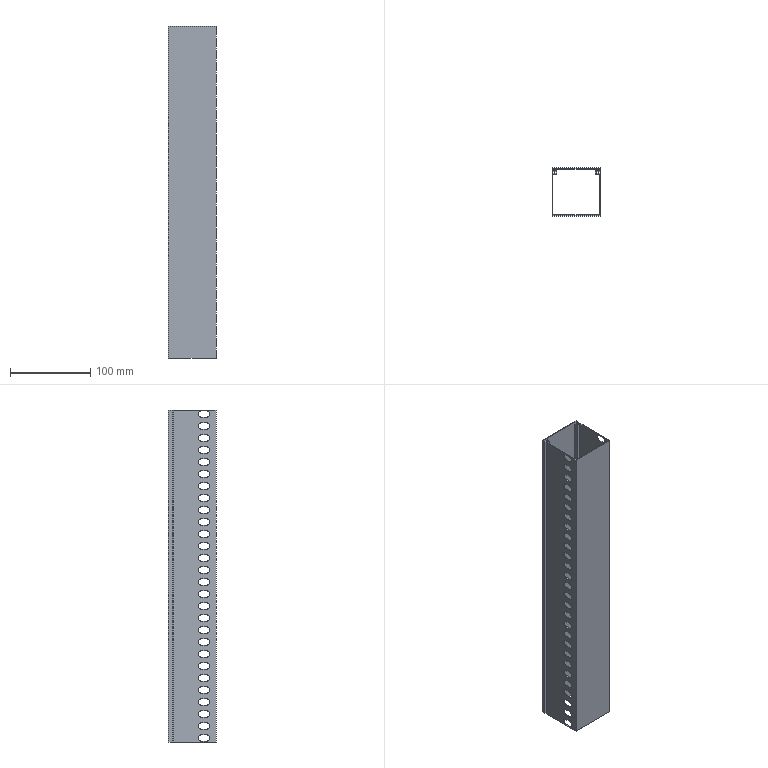Part | SolidWorks | features BaseBody 1 | 1 solid | 250 faces | box 60 x 60 x 415 mm | volume 100737 mm3 | plane 138 | cylinder 112 | commonest cylinder face diameters 8 x112